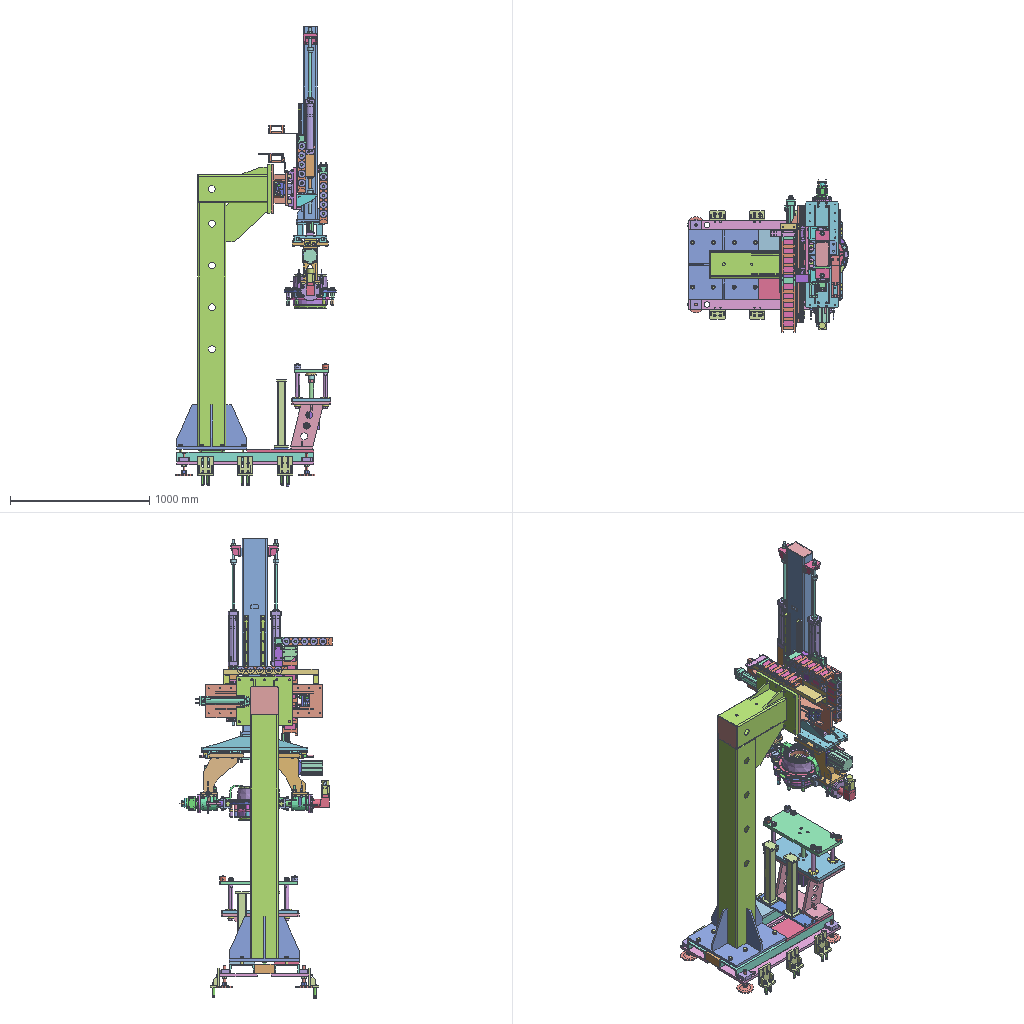Assembly | STEP file | 135 different items | 725 placed | box 1152 x 1093 x 3299 mm
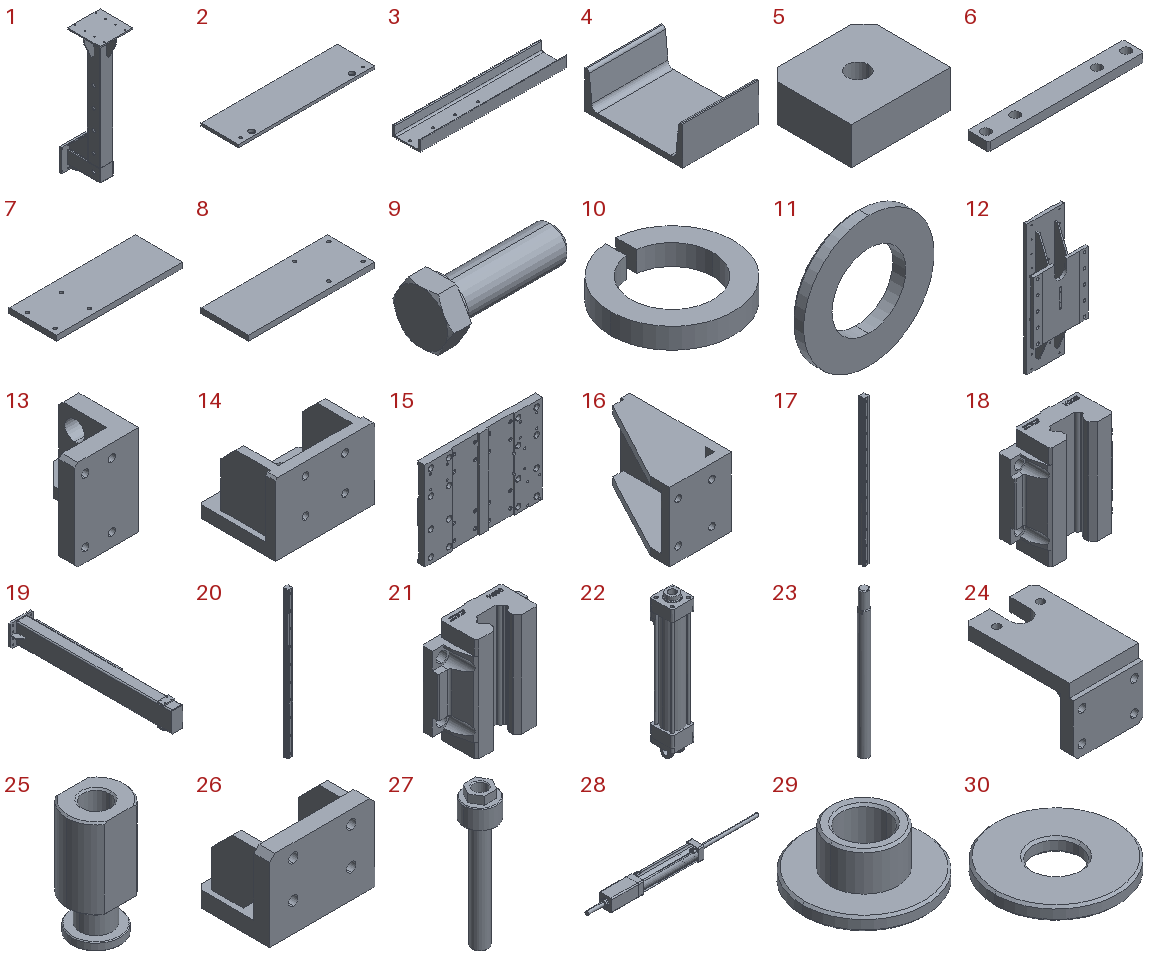Parts list (item | name | quantity | parent item | size | volume):
1 | YCD14007A-08.01.03 Column | x1 | in YCD14007A-08.01.00 Frame Component | 500 x 676 x 2044 mm | 25161780 mm3
2 | Base Plate | x2 | in YCD14007A-08.01.01 Base | 980 x 270 x 20 mm | 5232113 mm3
3 | 18# B Channel 980 (GB_INTERCHANGEABLE_PARTS_TM_SS 18X980)_GB_INTERCHANGEABLE_PARTS_TM_SS 18X980 | x2 | in YCD14007A-08.01.01 Base | 980 x 180 x 70 mm | 2864896 mm3
4 | 18# B Channel 140 (GB_INTERCHANGEABLE_PARTS_TM_SS 18X140)_GB_INTERCHANGEABLE_PARTS_TM_SS 18X140 | x2 | in YCD14007A-08.01.01 Base | 140 x 180 x 70 mm | 410063 mm3
5 | Thickening Block | x4 | in YCD14007A-08.01.01 Base | 80 x 70 x 30 mm | 157784 mm3
6 | Pad Plate | x1 | in YCD14007A-08.01.01 Base | 186 x 25 x 10 mm | 42619 mm3
7 | Small Pad Plate | x1 | in YCD14007A-08.01.01 Base | 480 x 180 x 20 mm | 1718952 mm3
8 | Small Pad Plate 1 | x1 | in YCD14007A-08.01.01 Base | 480 x 180 x 20 mm | 1718952 mm3
9 | Hex Head Bolt GB/T5783-2000 Fully Threaded M16x50 | x8 | in YCD14007A-08.01.00 Frame Component | 60 x 27.713 x 24 mm | 14933 mm3
10 | Spring Lock Washer GB/T93-1987 Standard Type (Assembly) 16x4.1 | x8 | in YCD14007A-08.01.00 Frame Component | 24.356 x 24.313 x 4.1 mm | 1031 mm3
11 | Flat Washer GB/T97.2-1985 Chamfered Type Grade A 16x3 | x8 | in YCD14007A-08.01.00 Frame Component | 30 x 3 x 30 mm | 1414 mm3
12 | YCD14007A-08.02.04-Lift Connecting Plate-A2 | x1 | in YCD14007A-08.02.00 Lifting Assembly | 350 x 120 x 840 mm | 6654945 mm3
13 | YCD14007A-08.02.07-Buffer Limit Seat-A3 | x1 | in YCD14007A-08.02.00 Lifting Assembly | 60 x 60 x 85 mm | 134562 mm3
14 | YCD14007A-08.02.08-Horizontal Cylinder Seat-A3 | x1 | in YCD14007A-08.02.00 Lifting Assembly | 100 x 77 x 72 mm | 177246 mm3
15 | YCD14007A-08.02.02-Adapter Plate-A3 | x1 | in YCD14007A-08.02.00 Lifting Assembly | 400 x 25 x 300 mm | 2208282 mm3
16 | YCD14007A-08.02.03-Lift Cylinder Seat-A3 | x2 | in YCD14007A-08.02.00 Lifting Assembly | 85 x 140.5 x 95 mm | 348010 mm3
17 | Slide Rail HGR35R840C | x2 | in Guide Rail Assembly | 34 x 29 x 840 mm | 682718 mm3
18 | HGW35CA20C+ZZ Slider | x4 | in Guide Rail Assembly | 100 x 40.5 x 112.7 mm | 283296 mm3
19 | YCD14007A-08.02.01 Slide | x1 | in YCD14007A-08.02.00 Lifting Assembly | 200 x 1406 x 200 mm | 5203563 mm3
20 | HGR30R-760 Slide Rail | x2 | in YCD14007A-08.02.00 Lifting Assembly | 28 x 26 x 760 mm | 438693 mm3
21 | HGW30 | x4 | in YCD14007A-08.02.00 Lifting Assembly | 90 x 36 x 97.7 mm | 189576 mm3
22 | MDBD50-250-A56 (Barrel) | x1 | in MBDB50-250-M9P | 65.01 x 74.997 x 403 mm | 1011039 mm3
23 | MDBD50-250-A56 (Rod) | x1 | in MBDB50-250-M9P | 20 x 20 x 309 mm | 94732 mm3
24 | YCD14007A-08.02.09-Horizontal Cylinder Connecting Plate-A3 | x1 | in YCD14007A-08.02.00 Lifting Assembly | 80 x 125 x 75 mm | 230135 mm3
25 | YCD14007A-08.02.11 Horizontal Cylinder Joint | x1 | in YCD14007A-08.02.00 Lifting Assembly | 36 x 30 x 71 mm | 47737 mm3
26 | YCD14007A-08.02.05-Lift Cylinder Connecting Plate-A3_Default<Machined> | x2 | in YCD14007A-08.02.00 Lifting Assembly | 100 x 70 x 75 mm | 222556 mm3
27 | YCD14007A-08.02.06-Extension Adjusting Rod-A4 | x4 | in YCD14007A-08.02.00 Lifting Assembly | 41 x 41 x 175 mm | 76364 mm3
28 | MDBB63-300-M9P_55_0_0 | x2 | in YCD14007A-08.02.00 Lifting Assembly | - | -
29 | YCD14007A-08.02.19 Lifting Cylinder Joint Modified | x3 | in YCD14007A-08.02.00 Lifting Assembly, Clamping Unit Assembly Left | 55 x 55 x 23 mm | 18397 mm3
30 | YCD14007A-08.02.19A Lifting Cylinder Joint Stop Plate Added | x3 | in YCD14007A-08.02.00 Lifting Assembly, Clamping Unit Assembly Left | 55 x 55 x 6 mm | 12037 mm3
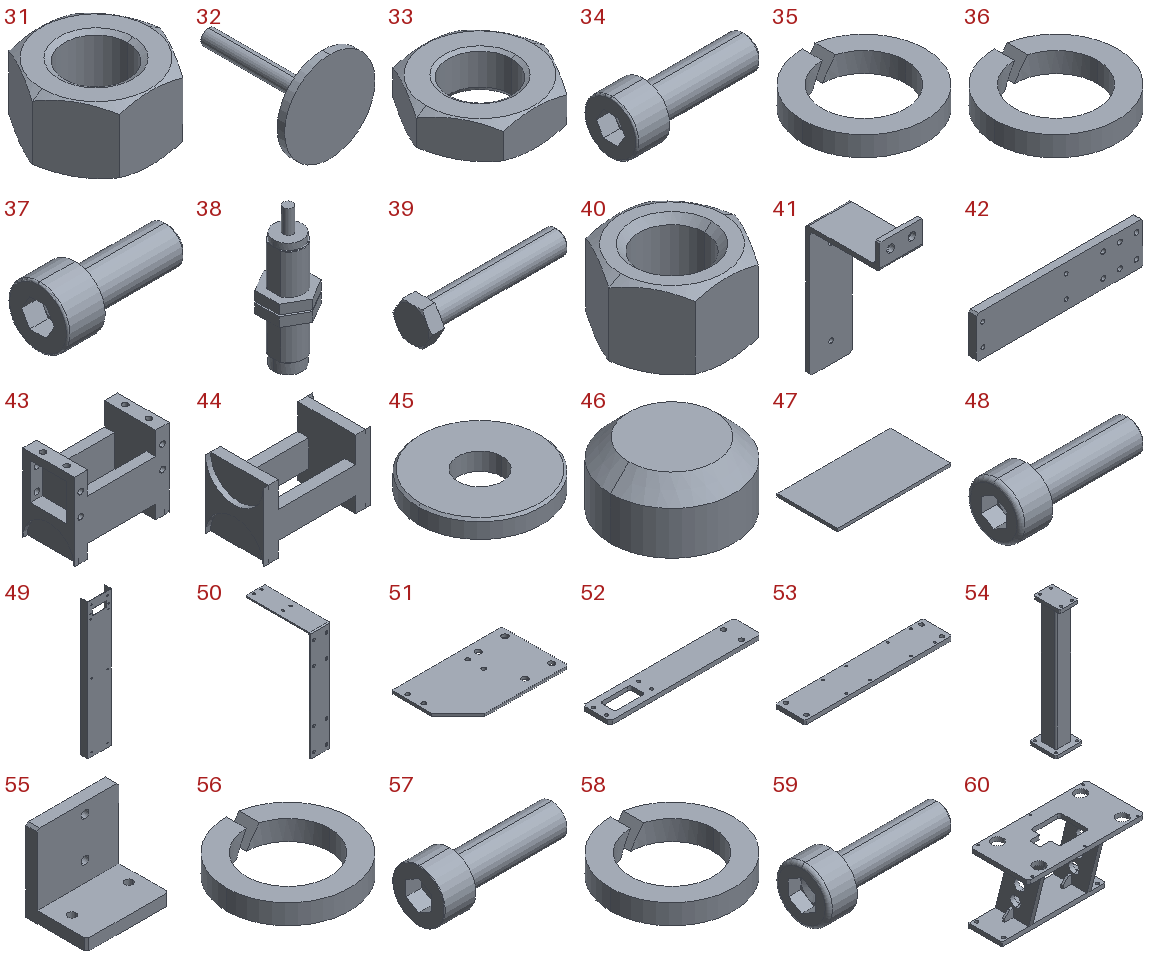31 | Hex Nut GB 6170-2000 M20 | x14 | in YCD14007A-08.02.00 Lifting Assembly, Clamping Unit Assembly Left | 34.641 x 30 x 18 mm | 9644 mm3
32 | Leveling Foot BF-20 | x4 | in Leveling Foot | 120 x 162 x 120 mm | 186987 mm3
33 | Hex Thin Nut M20_GB_FASTENER_NUT_STNAB B M20-N | x4 | in Leveling Foot | 34.641 x 30 x 10 mm | 5315 mm3
34 | Socket Head Cap Screw GB70.1-2000 M8X25 | x14 | in Turnover Unit Assembly, Clamping Unit Slide, Clamping Unit Assembly Left, Clamping Unit Assembly | 33 x 13 x 13 mm | 2167 mm3
35 | Spring Washer GB 93-87 10 | x32 | in Turnover Unit Assembly, Clamping Unit Assembly Left, Clamping Unit Assembly | 16.1 x 16.1 x 2.6 mm | 276.51 mm3
36 | Spring Washer GB 93-87 8 | x56 | in Turnover Unit Assembly, Clamping Unit Slide, Clamping Unit Assembly Left, Clamping Unit Assembly | 12.88 x 12.88 x 2.1 mm | 143.98 mm3
37 | Socket Head Cap Screw GB70.1-2000 M8X20 | x6 | in Turnover Unit Assembly | 28 x 13 x 13 mm | 1915 mm3
38 | Shock Absorber (SMC) RB2015 | x3 | in Turnover Unit Assembly, Clamping Unit Slide | 27 x 31.177 x 88.2 mm | 26039 mm3
39 | Hex Head Bolt GB5780-2000 M16(X1.5)X90_GB_FASTENER_BOLT_HHBFPT A M16X1.5X90-N | x3 | in Turnover Unit Assembly, Clamping Unit Slide | 99.82 x 27.332 x 23.67 mm | 22788 mm3
40 | Hex Nut GB 6170-2000 M16(X1.5)_GB_HEXAGON_TYPE10 M16X1.5-N | x6 | in Turnover Unit Assembly, Clamping Unit Slide | 27.713 x 24 x 16.4 mm | 5375 mm3
41 | Cable Carrier Channel Bracket | x3 | in Turnover Unit Assembly | 40 x 70 x 142 mm | 32841 mm3
42 | Cable Carrier Support Plate | x1 | in Cable Carrier Assembly | 180 x 8 x 45 mm | 63350 mm3
43 | Cable Carrier Part 1 | x4 | in Fully Enclosed Cable Carrier TLF-03 | 104 x 56 x 85 mm | 152286 mm3
44 | Cable Carrier Part 2 | x20 | in Fully Enclosed Cable Carrier TLF-03 | 104 x 56 x 66 mm | 123504 mm3
45 | Cable Carrier Part 3 | x40 | in Fully Enclosed Cable Carrier TLF-03 | 56 x 56 x 8 mm | 17104 mm3
46 | Cable Carrier Part 4 | x40 | in Fully Enclosed Cable Carrier TLF-03 | 20 x 20 x 10 mm | 2887 mm3
47 | Cable Carrier Seal Plate | x40 | in Fully Enclosed Cable Carrier TLF-03 | 75 x 40 x 2 mm | 6000 mm3
48 | Socket Head Cap Screw M5X16_GB_FASTENER_SCREWS_HSHCS M5X16-C | x8 | in Cable Carrier Assembly, Servo Motor SGMJV-04ADE6S and Reducer WPLE60-100 | 21 x 8.5 x 8.5 mm | 555.936 mm3
49 | Cable Carrier Channel | x1 | in Turnover Unit Assembly | 118 x 35 x 680 mm | 123926 mm3
50 | Cable Carrier Bracket | x1 | in Turnover Unit Assembly | 60 x 202 x 340 mm | 126408 mm3
51 | Cable Carrier Bracket 1 | x1 | in Turnover Unit Assembly | 165 x 100 x 4 mm | 61306 mm3
52 | Cable Carrier Bracket 2 | x1 | in Turnover Unit Assembly | 300 x 55 x 8 mm | 115449 mm3
53 | Fixed Base Plate | x1 | in Turnover Unit Assembly | 500 x 100 x 14 mm | 687217 mm3
54 | Cable Fixing Bracket | x2 | in Turnover Unit Assembly | 100 x 100 x 485 mm | 512449 mm3
55 | Cable Carrier Bracket 3 | x1 | in Turnover Unit Assembly | 72 x 53.558 x 72 mm | 81626 mm3
56 | Spring Washer GB 93-87 6 | x14 | in Turnover Unit Assembly, Clamping Unit Assembly Left, Clamping Unit Assembly | 9.88 x 9.88 x 1.6 mm | 64.217 mm3
57 | Socket Head Cap Screw GB/T70.1-2000 M6x20 | x14 | in Turnover Unit Assembly, YCD14007A-08.03.08 Left-Hand Mechanism.00, YCD14007A-08.03.07.00 Right-Hand Mechanism | 26 x 10 x 10 mm | 969.381 mm3
58 | Spring Washer 5_GB_FASTENER_WASHER_SW 5 | x8 | in Turnover Unit Assembly, Servo Motor SGMJV-04ADE6S and Reducer WPLE60-100 | 8 x 8 x 1.3 mm | 34.298 mm3
59 | _PreviewCfg | x2 | in Turnover Unit Assembly | 7.6 x 3 x 3 mm | 21.652 mm3
60 | Lifting Bracket | x1 | in Turnover Unit Assembly | 560 x 289.5 x 340 mm | 5840696 mm3
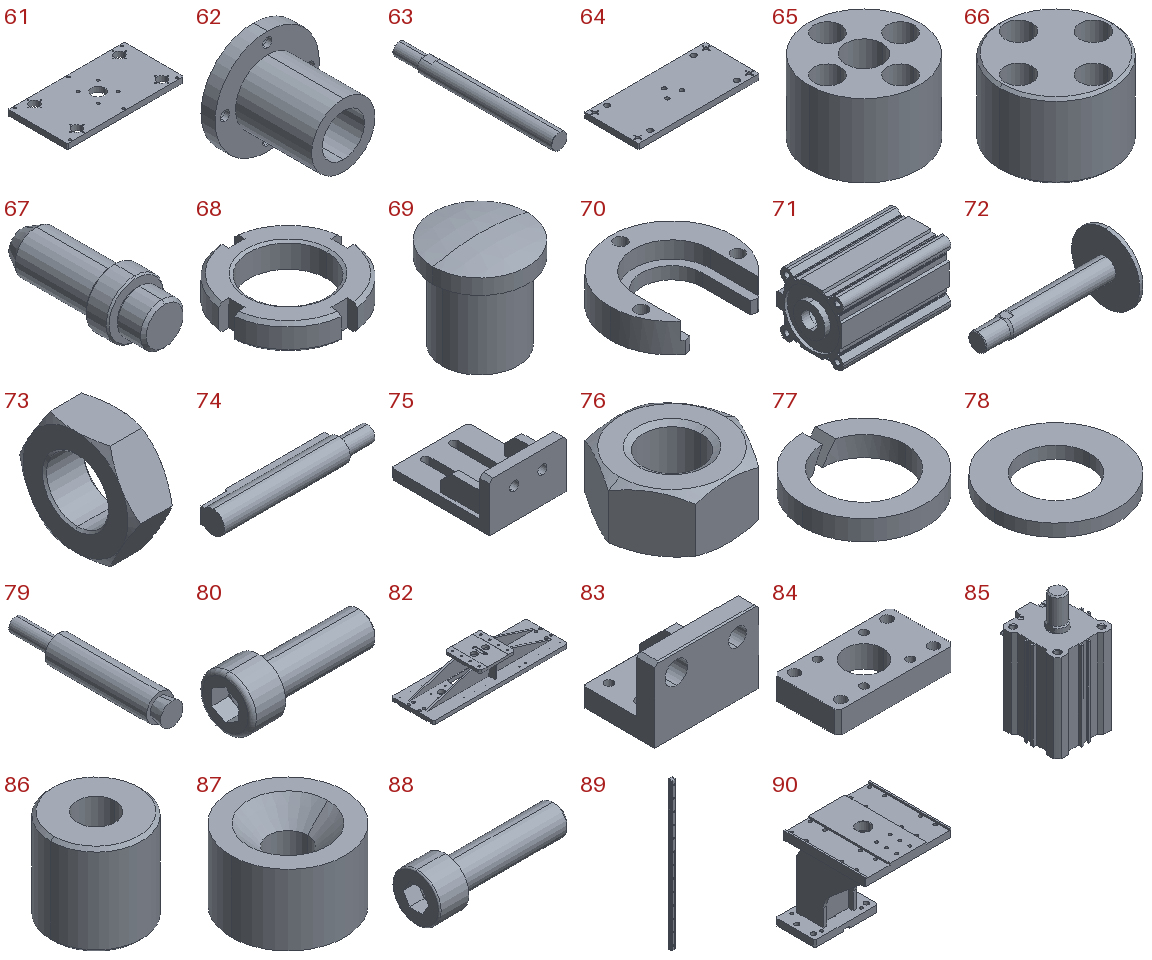61 | Lifting Base Plate | x1 | in Lift Positioning YCD14007A-17-0007-00 | 550 x 280 x 25 mm | 3578848 mm3
62 | LMF30UU | x4 | in Lift Positioning YCD14007A-17-0007-00 | 74 x 64 x 74 mm | 80630 mm3
63 | 30 Plain Shaft | x4 | in Lift Positioning YCD14007A-17-0007-00 | 30 x 305 x 30 mm | 202030 mm3
64 | Lifting Top Plate | x1 | in Lift Positioning YCD14007A-17-0007-00 | 560 x 250 x 25 mm | 3417013 mm3
65 | Locating Pin Seat | x2 | in Lift Positioning YCD14007A-17-0007-00 | 45 x 45 x 30 mm | 32214 mm3
66 | Locating Pin Seat | x2 | in Lift Positioning YCD14007A-17-0007-00 | 45 x 45 x 30 mm | 38603 mm3
67 | Locating Pin | x2 | in Lift Positioning YCD14007A-17-0007-00 | 20 x 50 x 20 mm | 9513 mm3
68 | Round Nut GB/T810-1988 M24x1.5 | x8 | in Lift Positioning YCD14007A-17-0007-00 | 37.67 x 37.67 x 8 mm | 4810 mm3
69 | Cylinder Joint | x1 | in Lift Positioning YCD14007A-17-0007-00 | 50 x 50 x 51 mm | 50075 mm3
70 | Cylinder Gland 2 | x1 | in Lift Positioning YCD14007A-17-0007-00 | 85 x 76.879 x 20 mm | 52737 mm3
71 | - | x1 | - | 205.5 x 123.5 x 117 mm | 1275384 mm3
72 | - | x1 | - | 193.5 x 100 x 100 mm | 165666 mm3
73 | NT-10(CQ2)_HI | x1 | - | 16 x 47.343 x 41 mm | 15625 mm3
74 | D_A96(CQ2L_100)_HI | x2 | - | 27 x 4.5 x 4 mm | 337.66 mm3
75 | Fixed Foot Plate | x6 | in Turnover Unit Assembly | 110 x 140 x 69 mm | 308717 mm3
76 | Nut M10-N_GB_FASTENER_NUT_SNAB1 M10-N | x12 | in Steel Expansion Bolt Assembly M10 | 18.475 x 16 x 8.4 mm | 1367 mm3
77 | Spring Washer SW 8_GB_FASTENER_WASHER_SW 8 | x12 | in Steel Expansion Bolt Assembly M10 | 12.88 x 12.88 x 2.1 mm | 143.98 mm3
78 | Flat Washer 10_GB_FASTENER_WASHER_SMWC 10 | x12 | in Steel Expansion Bolt Assembly M10 | 20 x 20 x 2 mm | 438.252 mm3
79 | Expansion Bolt M10X110 | x12 | in Steel Expansion Bolt Assembly M10 | 19.178 x 110 x 19.178 mm | 19450 mm3
80 | Socket Head Cap Screw M10X30-N_GB_FASTENER_SCREWS_HSHCS M10X30-N | x12 | in Turnover Unit Assembly | 40 x 16 x 16 mm | 4032 mm3
81 | Part 7 | x1 | in OP70 | - | -
82 | YCD14007A-08.03.02 Clamping Slide | x1 | in Clamping Unit Slide | 760 x 240 x 115 mm | 4249230 mm3
83 | YCD14007A-08.03.01 Buffer Limit Seat | x2 | in Clamping Unit Slide | 85 x 60 x 60 mm | 134508 mm3
84 | Locking Cylinder Mounting Plate | x1 | in Clamping Unit Slide | 100 x 56 x 19 mm | 79159 mm3
85 | A_CDQ2A40-40DM-A96V(0) | x2 | in Clamping Unit Slide, Latch Pin Assembly | 52 x 66.1 x 108 mm | 193246 mm3
86 | Locking Cylinder Joint | x1 | in Clamping Unit Slide | 30 x 30 x 30 mm | 16100 mm3
87 | Clamping Pad | x1 | in Clamping Unit Slide | 16 x 16 x 10 mm | 1679 mm3
88 | Socket Head Cap Screw GB70.1-2000 M8X30 | x38 | in Clamping Unit Slide, Clamping Unit Assembly Left, Clamping Unit Assembly | 38 x 13 x 13 mm | 2418 mm3
89 | HGR25R760C Guide Rail | x2 | in Clamping Unit Slide | 23 x 22 x 760 mm | 316727 mm3
90 | YCD14007A-08.03.06 Clamping Arm (Left) | x1 | in Clamping Unit Assembly Left | 260 x 306 x 295 mm | 2759054 mm3
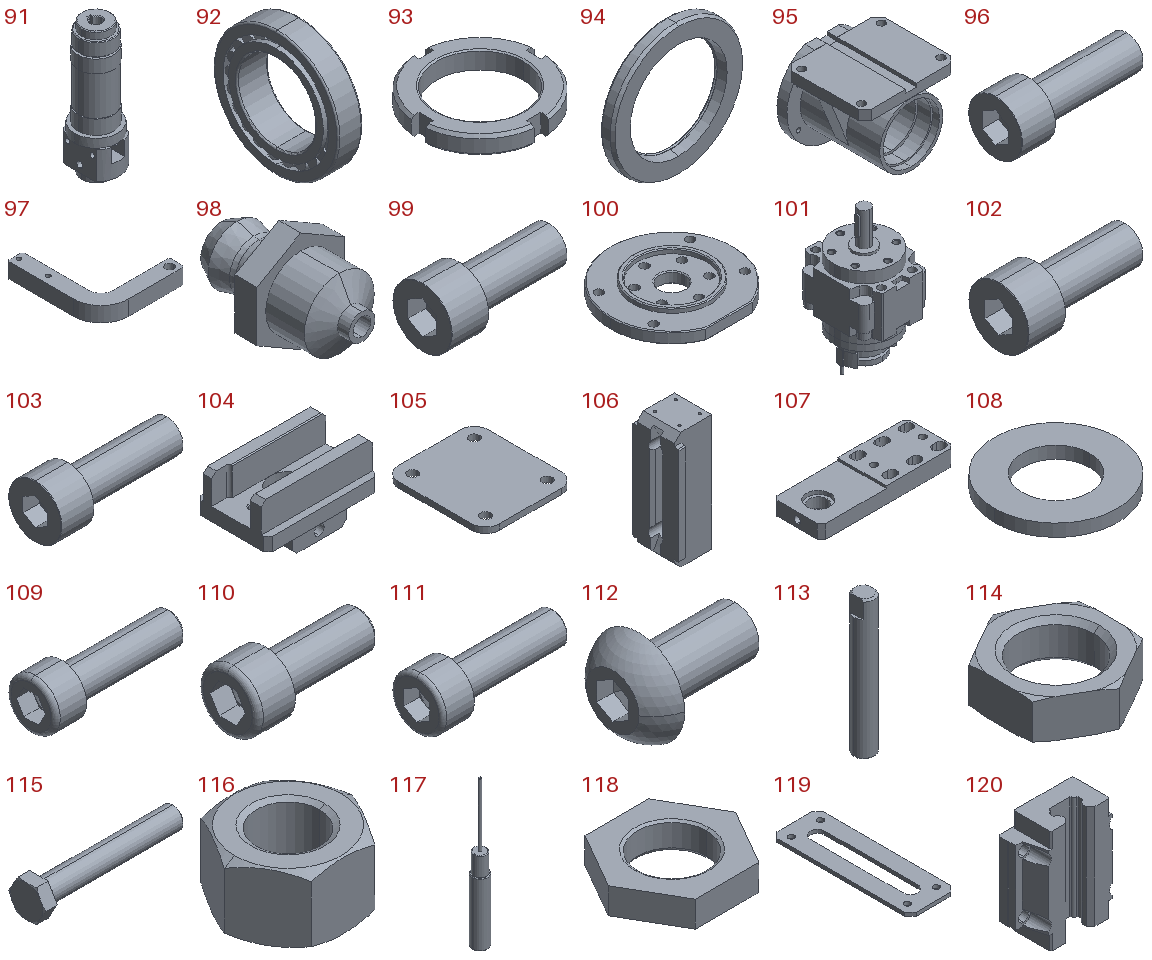91 | YCD14007A-08.03.08.01 Shaft (Cylinder) | x1 | in YCD14007A-08.03.08 Left-Hand Mechanism.00 | 60 x 65 x 185 mm | 338320 mm3
92 | Tapered Roller Bearing GB/T297-94 32010 | x4 | in YCD14007A-08.03.08 Left-Hand Mechanism.00, YCD14007A-08.03.07.00 Right-Hand Mechanism | 20 x 80 x 80 mm | 43880 mm3
93 | Round Nut GB/T810-1988 M48x1.5 | x2 | in YCD14007A-08.03.08 Left-Hand Mechanism.00 | 67.528 x 67.528 x 10 mm | 16343 mm3
94 | Lip Seal GB/T13871.1-2007 Type B B58_B1 | x3 | in YCD14007A-08.03.08 Left-Hand Mechanism.00, YCD14007A-08.03.07.00 Right-Hand Mechanism | 85 x 8 x 85 mm | 12919 mm3
95 | YCD14007A-08.03.07.04 Bearing Seat | x2 | in YCD14007A-08.03.08 Left-Hand Mechanism.00, YCD14007A-08.03.07.00 Right-Hand Mechanism | 140 x 135 x 130 mm | 675590 mm3
96 | Socket Head Cap Screw GB/T70.1-2000 M10x30 | x4 | in YCD14007A-08.03.08 Left-Hand Mechanism.00, YCD14007A-08.03.07.00 Right-Hand Mechanism | 40 x 16 x 16 mm | 4081 mm3
97 | YCD14007A-08.03.07.06 Limit Rod | x2 | in YCD14007A-08.03.08 Left-Hand Mechanism.00, YCD14007A-08.03.07.00 Right-Hand Mechanism | 100 x 112 x 18 mm | 57197 mm3
98 | Straight Grease Fitting JB/T7940.1-1995 8 | x2 | in YCD14007A-08.03.08 Left-Hand Mechanism.00, YCD14007A-08.03.07.00 Right-Hand Mechanism | 10 x 16 x 11.547 mm | 627.523 mm3
99 | Socket Head Cap Screw GB/T70.1-2000 M10x25 | x8 | in YCD14007A-08.03.08 Left-Hand Mechanism.00, YCD14007A-08.03.07.00 Right-Hand Mechanism | 35 x 16 x 16 mm | 3688 mm3
100 | YCD14007A-08.03.08.02 Adapter Flange (Cylinder) | x1 | in YCD14007A-08.03.08 Left-Hand Mechanism.00 | 135 x 130 x 17 mm | 160209 mm3
101 | CDRB1BW63-180S-S79_A_0 | x1 | in YCD14007A-08.03.08 Left-Hand Mechanism.00 | - | -
102 | Socket Head Cap Screw GB/T70.1-2000 M8x20 | x6 | in YCD14007A-08.03.08 Left-Hand Mechanism.00 | 28 x 13 x 13 mm | 1937 mm3
103 | Socket Head Cap Screw GB/T70.1-2000 M8x25 | x8 | in YCD14007A-08.03.08 Left-Hand Mechanism.00, YCD14007A-08.03.07.00 Right-Hand Mechanism | 33 x 13 x 13 mm | 2189 mm3
104 | YCD14007A-08.03.07.08 Gripper Seat | x2 | in YCD14007A-08.03.08 Left-Hand Mechanism.00, YCD14007A-08.03.07.00 Right-Hand Mechanism | 125 x 80 x 67 mm | 253618 mm3
105 | YCD14007A-08.03.08.05 Engraving Plate | x2 | in Clamping Unit Assembly Left, Clamping Unit Assembly | 32 x 36 x 2 mm | 2184 mm3
106 | Nylon Claw M20 | x2 | in Clamping Unit Assembly Left, Clamping Unit Assembly | 40 x 50 x 125 mm | 179842 mm3
107 | YCD14007A-08.02.17 Lock Plate | x1 | in Clamping Unit Assembly Left | 165 x 60 x 20 mm | 154509 mm3
108 | Flat Washer GB 95-85 10_GB_FASTENER_WASHER_SMWC 10 | x4 | in Clamping Unit Assembly Left | 20 x 20 x 2 mm | 438.252 mm3
109 | Socket Head Cap Screw GB70.1-2000 M10X35 | x12 | in Clamping Unit Assembly Left, Clamping Unit Assembly | 45 x 16 x 16 mm | 4402 mm3
110 | Socket Head Cap Screw GB70.1-2000 M10X25 | x4 | in Clamping Unit Assembly Left, Clamping Unit Assembly | 35 x 16 x 16 mm | 3616 mm3
111 | Socket Set Screw GB79-2000 M6X20_GB_FASTENER_SCREWS_HSHCS M6X20-N | x8 | in Clamping Unit Assembly Left, Clamping Unit Assembly | 26 x 10 x 10 mm | 958.089 mm3
112 | Socket Button Head Screw M3X6-N_GB_SOCKET_TYPE7 M3X6-N | x8 | in Clamping Unit Assembly Left, Clamping Unit Assembly | 7.65 x 5.7 x 5.7 mm | 68.602 mm3
113 | YCD14007A-08-03.07.07 Sensing Rod | x2 | in Clamping Unit Assembly Left, YCD14007A-08.03.07.00 Right-Hand Mechanism | 12 x 12 x 82 mm | 9083 mm3
114 | Hex Nut GB/T6172.1-2000 Grade A and B M12 | x4 | in Clamping Unit Assembly Left, YCD14007A-08.03.07.00 Right-Hand Mechanism, Clamping Unit Assembly | 17.386 x 20.03 x 6 mm | 858.5 mm3
115 | Hex Head Bolt GB5780-2000 M16X100 | x4 | in Clamping Unit Assembly Left, Clamping Unit Assembly | 110 x 27.713 x 24 mm | 24997 mm3
116 | Hex Nut GB 6170-2000 M16 | x8 | in Clamping Unit Assembly Left, Clamping Unit Assembly | 27.713 x 24 x 14.8 mm | 5071 mm3
117 | YB Inductive Proximity Switch | x6 | in Proximity Switch Assembly, Clamping Unit Assembly Left, Clamping Unit Assembly | 12 x 12 x 115 mm | 6984 mm3
118 | Fine-Thread Nut M12X1_GB_FASTENER_NUT_STNABTT M12X1.25-N | x14 | in Proximity Switch Assembly, Clamping Unit Assembly Left, Clamping Unit Assembly | 19.63 x 17 x 4 mm | 641.848 mm3
119 | Mounting Plate | x1 | in Proximity Switch Assembly | 40 x 120 x 3 mm | 10646 mm3
120 | HGW25CA0C+ZZ | x8 | in Clamping Unit Assembly Left, Clamping Unit Assembly | 70 x 30.5 x 82 mm | 109676 mm3
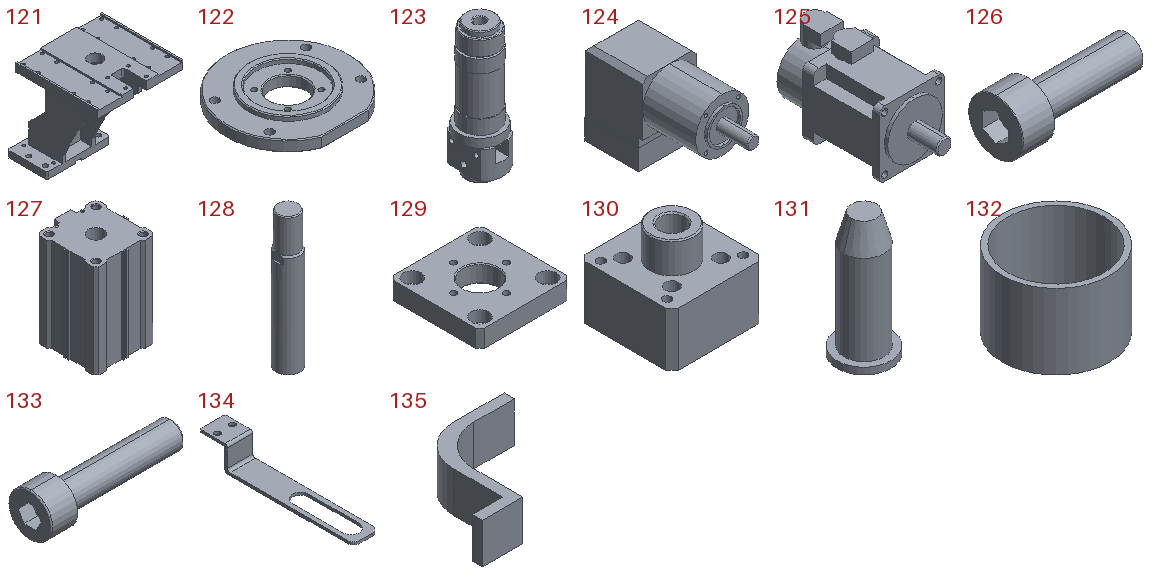121 | YCD14007A-08.03.03 Clamping Arm (Right) | x1 | in Clamping Unit Assembly | 260 x 306 x 295 mm | 2644303 mm3
122 | YCD14007A-08.03.07.05 Adapter Flange (Motor) | x1 | in YCD14007A-08.03.07.00 Right-Hand Mechanism | 135 x 130 x 17 mm | 158776 mm3
123 | YCD14007A-08.03.07.03 Shaft (Motor) | x1 | in YCD14007A-08.03.07.00 Right-Hand Mechanism | 60 x 65 x 185 mm | 341019 mm3
124 | Right-Angle Reducer WPLE60-100 | x1 | in Servo Motor SGMJV-04ADE6S and Reducer WPLE60-100 | 60.05 x 160.025 x 93 mm | 504170 mm3
125 | SGMJV-04ADE6S (Yaskawa Servo 0.4KW) | x1 | in Servo Motor SGMJV-04ADE6S and Reducer WPLE60-100 | 60 x 129 x 73 mm | 298777 mm3
126 | Socket Head Cap Screw GB/T70.1-2000 M5x16 | x4 | in YCD14007A-08.03.07.00 Right-Hand Mechanism | 21 x 8.5 x 8.5 mm | 561.928 mm3
127 | A_CDQ2A80-100DM-F9NV (Barrel) | x1 | in CDQ2A80-100DMZ | 98 x 108.4 x 153.5 mm | 1262277 mm3
128 | A_CDQ2A80-100DM-F9NV (Rod) | x1 | in CDQ2A80-100DMZ | 25 x 25 x 144.5 mm | 66720 mm3
129 | Clamping Cylinder Mounting Plate | x1 | in Clamping Unit Assembly | 104 x 104 x 20 mm | 167084 mm3
130 | YCD14007A-08.02.14 Latch Cylinder Seat | x1 | in Latch Pin Assembly | 76 x 76 x 69 mm | 233677 mm3
131 | YCD14007A-08.02.15 Latch Cylinder Joint | x1 | in Latch Pin Assembly | 24 x 24 x 55 mm | 9061 mm3
132 | Oil-Free Bushing JH-B-18-14 | x2 | in Latch Pin Assembly | 20 x 20 x 14 mm | 835.664 mm3
133 | Socket Head Cap Screw GB70.1-2000 M8X35 | x4 | in Clamping Unit Assembly | 43 x 13 x 13 mm | 2669 mm3
134 | Proximity Switch Bracket | x2 | in Clamping Unit Assembly | 20 x 122 x 20 mm | 4207 mm3
135 | Pressure Rod | x2 | in Turnover Unit Assembly | 120 x 98.5 x 40 mm | 83400 mm3
Placements (level | parent | child | x y z in mm | rotation matrix by rows), first 157 of 765 lines:
1 | Turnover Unit Assembly | YCD14007A-08.01.00 Frame Component | -651.902 -316.685 -698.035 | 0 1 0 1 0 0 0 0 -1
2 | YCD14007A-08.01.00 Frame Component | YCD14007A-08.01.03 Column | -109.585 -100.226 1002.0 | 1 0 0 0 1 0 0 0 1
2 | YCD14007A-08.01.00 Frame Component | YCD14007A-08.01.01 Base | -386.402 100.206 1132.0 | 0 1 0 1 0 0 0 0 -1
3 | YCD14007A-08.01.01 Base | Base Plate | 39.567 91.817 -0.0 | 1 0 0 0 1 0 0 0 1
3 | YCD14007A-08.01.01 Base | 18# B Channel 980 (GB_INTERCHANGEABLE_PARTS_TM_SS 18X980)_GB_INTERCHANGEABLE_PARTS_TM_SS 18X980 | -450.433 116.817 90.0 | 1 0 0 0 -1 0 0 0 -1
3 | YCD14007A-08.01.01 Base | 18# B Channel 980 (GB_INTERCHANGEABLE_PARTS_TM_SS 18X980)_GB_INTERCHANGEABLE_PARTS_TM_SS 18X980 | -450.433 436.817 90.0 | 1 0 0 0 -1 0 0 0 -1
3 | YCD14007A-08.01.01 Base | Base Plate | 39.567 461.817 20.0 | 1 0 0 0 -1 0 0 0 -1
3 | YCD14007A-08.01.01 Base | 18# B Channel 140 (GB_INTERCHANGEABLE_PARTS_TM_SS 18X140)_GB_INTERCHANGEABLE_PARTS_TM_SS 18X140 | -360.433 206.816 90.0 | 0 1 0 1 0 0 0 0 -1
3 | YCD14007A-08.01.01 Base | 18# B Channel 140 (GB_INTERCHANGEABLE_PARTS_TM_SS 18X140)_GB_INTERCHANGEABLE_PARTS_TM_SS 18X140 | 439.567 206.816 90.0 | 0 1 0 1 0 0 0 0 -1
3 | YCD14007A-08.01.01 Base | Thickening Block | -400.433 561.817 20.0 | 0.9999 0.01671 0 -0.01671 0.9999 0 0 0 1
3 | YCD14007A-08.01.01 Base | Thickening Block | 479.567 561.817 50.0 | -1 0 0 0 1 0 0 0 -1
3 | YCD14007A-08.01.01 Base | Thickening Block | -400.433 -8.184 50.0 | 1 0 0 0 -1 0 0 0 -1
3 | YCD14007A-08.01.01 Base | Thickening Block | 479.567 -8.184 50.0 | 1 0 0 0 -1 0 0 0 -1
3 | YCD14007A-08.01.01 Base | Pad Plate | -200.433 276.817 90.0 | 1 0 0 0 1 0 0 0 1
3 | YCD14007A-08.01.01 Base | Small Pad Plate | 289.567 116.817 90.0 | -1 0 0 0 -1 0 0 0 1
3 | YCD14007A-08.01.01 Base | Small Pad Plate 1 | 289.567 436.817 90.0 | 1 0 0 0 1 0 0 0 1
2 | YCD14007A-08.01.00 Frame Component | Hex Head Bolt GB/T5783-2000 Fully Threaded M16x50 | 50.415 -325.226 984.9 | 0 0 -1 0 1 0 1 0 0
2 | YCD14007A-08.01.00 Frame Component | Spring Lock Washer GB/T93-1987 Standard Type (Assembly) 16x4.1 | 50.415 -325.226 994.9 | 1 0 0 0 1 0 0 0 1
2 | YCD14007A-08.01.00 Frame Component | Flat Washer GB/T97.2-1985 Chamfered Type Grade A 16x3 | 50.415 -325.226 1010.644 | 1 0 0 0 0 1 0 -1 -0
2 | YCD14007A-08.01.00 Frame Component | Spring Lock Washer GB/T93-1987 Standard Type (Assembly) 16x4.1 | -269.585 -325.226 994.9 | 1 0 0 0 1 0 0 0 1
2 | YCD14007A-08.01.00 Frame Component | Spring Lock Washer GB/T93-1987 Standard Type (Assembly) 16x4.1 | 50.415 -175.226 994.9 | 1 0 0 0 1 0 0 0 1
2 | YCD14007A-08.01.00 Frame Component | Spring Lock Washer GB/T93-1987 Standard Type (Assembly) 16x4.1 | -269.585 -175.226 994.9 | 1 0 0 0 1 0 0 0 1
2 | YCD14007A-08.01.00 Frame Component | Spring Lock Washer GB/T93-1987 Standard Type (Assembly) 16x4.1 | 50.415 -25.226 994.9 | 1 0 0 0 1 0 0 0 1
2 | YCD14007A-08.01.00 Frame Component | Spring Lock Washer GB/T93-1987 Standard Type (Assembly) 16x4.1 | -269.585 -25.226 994.9 | 1 0 0 0 1 0 0 0 1
2 | YCD14007A-08.01.00 Frame Component | Spring Lock Washer GB/T93-1987 Standard Type (Assembly) 16x4.1 | 50.415 124.774 994.9 | 1 0 0 0 1 0 0 0 1
2 | YCD14007A-08.01.00 Frame Component | Spring Lock Washer GB/T93-1987 Standard Type (Assembly) 16x4.1 | -269.585 124.774 994.9 | 1 0 0 0 1 0 0 0 1
2 | YCD14007A-08.01.00 Frame Component | Flat Washer GB/T97.2-1985 Chamfered Type Grade A 16x3 | -269.585 -325.226 1010.644 | 1 0 0 0 0 1 0 -1 -0
2 | YCD14007A-08.01.00 Frame Component | Flat Washer GB/T97.2-1985 Chamfered Type Grade A 16x3 | 50.415 -175.226 1010.644 | 1 0 0 0 0 1 0 -1 -0
2 | YCD14007A-08.01.00 Frame Component | Flat Washer GB/T97.2-1985 Chamfered Type Grade A 16x3 | -269.585 -175.226 1010.644 | 1 0 0 0 0 1 0 -1 -0
2 | YCD14007A-08.01.00 Frame Component | Flat Washer GB/T97.2-1985 Chamfered Type Grade A 16x3 | 50.415 -25.226 1010.644 | 1 0 0 0 0 1 0 -1 -0
2 | YCD14007A-08.01.00 Frame Component | Flat Washer GB/T97.2-1985 Chamfered Type Grade A 16x3 | -269.585 -25.226 1010.644 | 1 0 0 0 0 1 0 -1 -0
2 | YCD14007A-08.01.00 Frame Component | Flat Washer GB/T97.2-1985 Chamfered Type Grade A 16x3 | 50.415 124.774 1010.644 | 1 0 0 0 0 1 0 -1 -0
2 | YCD14007A-08.01.00 Frame Component | Flat Washer GB/T97.2-1985 Chamfered Type Grade A 16x3 | -269.585 124.774 1010.644 | 1 0 0 0 0 1 0 -1 -0
2 | YCD14007A-08.01.00 Frame Component | Hex Head Bolt GB/T5783-2000 Fully Threaded M16x50 | -269.585 -325.226 984.9 | 0 0 -1 0 1 0 1 0 0
2 | YCD14007A-08.01.00 Frame Component | Hex Head Bolt GB/T5783-2000 Fully Threaded M16x50 | 50.415 -175.226 984.9 | 0 0 -1 0 1 0 1 0 0
2 | YCD14007A-08.01.00 Frame Component | Hex Head Bolt GB/T5783-2000 Fully Threaded M16x50 | -269.585 -175.226 984.9 | 0 0 -1 0 1 0 1 0 0
2 | YCD14007A-08.01.00 Frame Component | Hex Head Bolt GB/T5783-2000 Fully Threaded M16x50 | 50.415 -25.226 984.9 | 0 0 -1 0 1 0 1 0 0
2 | YCD14007A-08.01.00 Frame Component | Hex Head Bolt GB/T5783-2000 Fully Threaded M16x50 | -269.585 -25.226 984.9 | 0 0 -1 0 1 0 1 0 0
2 | YCD14007A-08.01.00 Frame Component | Hex Head Bolt GB/T5783-2000 Fully Threaded M16x50 | 50.415 124.774 984.9 | 0 0 -1 0 1 0 1 0 0
2 | YCD14007A-08.01.00 Frame Component | Hex Head Bolt GB/T5783-2000 Fully Threaded M16x50 | -269.585 124.774 984.9 | 0 0 -1 0 1 0 1 0 0
1 | Turnover Unit Assembly | YCD14007A-08.02.00 Lifting Assembly | -1012.217 -846.27 -316.467 | -0.8169 0.5767 0 0 0 -1 -0.5767 -0.8169 -0
2 | YCD14007A-08.02.00 Lifting Assembly | YCD14007A-08.02.04-Lift Connecting Plate-A2 | -918.783 78.885 0.0 | -0.5767 -0.8169 0 -0.8169 0.5767 0 0 0 -1
2 | YCD14007A-08.02.00 Lifting Assembly | YCD14007A-08.02.07-Buffer Limit Seat-A3 | -890.221 110.745 -132.161 | 0 0.8169 -0.5767 0 -0.5767 -0.8169 -1 0 -0
2 | YCD14007A-08.02.00 Lifting Assembly | YCD14007A-08.02.08-Horizontal Cylinder Seat-A3 | -879.161 50.914 -515.5 | 0.5767 0.8169 0 0.8169 -0.5767 0 0 0 -1
2 | YCD14007A-08.02.00 Lifting Assembly | YCD14007A-08.02.02-Adapter Plate-A3 | -881.701 236.317 -489.348 | 0 0.8169 0.5767 0 -0.5767 0.8169 1 0 0
2 | YCD14007A-08.02.00 Lifting Assembly | YCD14007A-08.02.03-Lift Cylinder Seat-A3 | -915.269 231.249 -594.348 | -0.5767 -0.8169 0 -0.8169 0.5767 0 0 0 -1
2 | YCD14007A-08.02.00 Lifting Assembly | YCD14007A-08.02.03-Lift Cylinder Seat-A3 | -915.269 231.249 -289.348 | -0.5767 -0.8169 0 -0.8169 0.5767 0 0 0 -1
2 | YCD14007A-08.02.00 Lifting Assembly | Guide Rail Assembly | -1028.88 -38.564 -420.0 | -0.5767 -0.8169 0 -0.8169 0.5767 0 0 0 -1
3 | Guide Rail Assembly | Slide Rail HGR35R840C | -69.443 -2.709 420.0 | 1 0 0 0 1 0 0 0 1
3 | Guide Rail Assembly | HGW35CA20C+ZZ Slider | -69.443 11.791 218.148 | 1 0 0 0 1 0 0 0 1
3 | Guide Rail Assembly | HGW35CA20C+ZZ Slider | -69.443 11.791 -79.452 | 1 0 0 0 1 0 0 0 1
2 | YCD14007A-08.02.00 Lifting Assembly | Guide Rail Assembly | -925.071 108.487 -420.0 | -0.5767 -0.8169 0 -0.8169 0.5767 0 0 0 -1
3 | Guide Rail Assembly | Slide Rail HGR35R840C | -69.443 -2.709 420.0 | 1 0 0 0 1 0 0 0 1
3 | Guide Rail Assembly | HGW35CA20C+ZZ Slider | -69.443 11.791 218.148 | 1 0 0 0 1 0 0 0 1
3 | Guide Rail Assembly | HGW35CA20C+ZZ Slider | -69.443 11.791 -79.452 | 1 0 0 0 1 0 0 0 1
2 | YCD14007A-08.02.00 Lifting Assembly | YCD14007A-08.02.01 Slide | -925.596 364.007 -589.348 | 0.8169 0.5767 0 -0.5767 0.8169 0 0 0 1
2 | YCD14007A-08.02.00 Lifting Assembly | HGR30R-760 Slide Rail | -910.626 258.633 -549.348 | 0 0.8169 -0.5767 0 -0.5767 -0.8169 -1 0 -0
2 | YCD14007A-08.02.00 Lifting Assembly | HGW30 | -1045.828 44.572 -549.348 | 0 0.8169 -0.5767 0 -0.5767 -0.8169 -1 0 -0
2 | YCD14007A-08.02.00 Lifting Assembly | HGW30 | -928.985 210.085 -549.348 | 0 0.8169 -0.5767 0 -0.5767 -0.8169 -1 0 -0
2 | YCD14007A-08.02.00 Lifting Assembly | HGR30R-760 Slide Rail | -910.626 258.633 -429.348 | 0 0.8169 -0.5767 0 -0.5767 -0.8169 -1 0 -0
2 | YCD14007A-08.02.00 Lifting Assembly | HGW30 | -1045.828 44.572 -429.348 | 0 0.8169 -0.5767 0 -0.5767 -0.8169 -1 0 -0
2 | YCD14007A-08.02.00 Lifting Assembly | HGW30 | -928.985 210.085 -429.348 | 0 0.8169 -0.5767 0 -0.5767 -0.8169 -1 0 -0
2 | YCD14007A-08.02.00 Lifting Assembly | MBDB50-250-M9P | -914.55 -16.727 -715.001 | -0.5767 0.8169 0 -0.8169 -0.5767 0 0 0 1
3 | MBDB50-250-M9P | MDBD50-250-A56 (Barrel) | -75.668 -3.348 187.501 | 1 0 0 0 1 0 0 0 1
3 | MBDB50-250-M9P | MDBD50-250-A56 (Rod) | -75.668 -3.348 219.653 | -0.6044 0.7967 0 -0.7967 -0.6044 0 0 0 1
2 | YCD14007A-08.02.00 Lifting Assembly | YCD14007A-08.02.09-Horizontal Cylinder Connecting Plate-A3 | -904.895 69.08 -396.848 | 0.5767 0.8169 0 0.8169 -0.5767 0 0 0 -1
2 | YCD14007A-08.02.00 Lifting Assembly | YCD14007A-08.02.11 Horizontal Cylinder Joint | -873.647 47.021 -391.348 | -0.6292 0.7773 0 0.7773 0.6292 0 0 0 -1
2 | YCD14007A-08.02.00 Lifting Assembly | YCD14007A-08.02.05-Lift Cylinder Connecting Plate-A3_Default<Machined> | -1689.456 -718.037 -351.848 | -0.8169 0 0.5767 0.5767 0 0.8169 0 1 -0
2 | YCD14007A-08.02.00 Lifting Assembly | YCD14007A-08.02.05-Lift Cylinder Connecting Plate-A3_Default<Machined> | -1689.456 -718.037 -626.848 | 0.8169 0 0.5767 -0.5767 0 0.8169 0 -1 0
2 | YCD14007A-08.02.00 Lifting Assembly | YCD14007A-08.02.06-Extension Adjusting Rod-A4 | -1642.333 -652.153 -336.848 | 0.8166 -0.0243 0.5767 -0.5765 0.01716 0.8169 -0.02975 -0.9996 -0
2 | YCD14007A-08.02.00 Lifting Assembly | YCD14007A-08.02.06-Extension Adjusting Rod-A4 | -1642.333 -652.153 -641.848 | 0.1425 0.8044 0.5767 -0.1006 -0.5679 0.8169 0.9847 -0.1744 -0
2 | YCD14007A-08.02.00 Lifting Assembly | MDBB63-300-M9P_55_0_0 | -1201.146 -27.19 -336.848 | -0.5767 0 -0.8169 -0.8169 0 0.5767 0 1 -0
2 | YCD14007A-08.02.00 Lifting Assembly | MDBB63-300-M9P_55_0_0 | -1201.146 -27.19 -641.848 | -0.5767 0 0.8169 -0.8169 0 -0.5767 0 -1 0
2 | YCD14007A-08.02.00 Lifting Assembly | YCD14007A-08.02.06-Extension Adjusting Rod-A4 | -1036.782 205.639 -641.848 | 0.1342 -0.8059 -0.5767 -0.09471 0.5689 -0.8169 0.9864 0.1642 0
2 | YCD14007A-08.02.00 Lifting Assembly | YCD14007A-08.02.06-Extension Adjusting Rod-A4 | -1036.782 205.639 -336.848 | -0.7262 -0.3742 -0.5767 0.5127 0.2642 -0.8169 0.458 -0.8889 0
2 | YCD14007A-08.02.00 Lifting Assembly | YCD14007A-08.02.19 Lifting Cylinder Joint Modified | -1030.15 215.034 -641.848 | -0.1862 0.7955 0.5767 0.1314 -0.5615 0.8169 0.9737 0.2279 -0
2 | YCD14007A-08.02.00 Lifting Assembly | YCD14007A-08.02.19A Lifting Cylinder Joint Stop Plate Added | -1021.787 226.88 -641.848 | 0.6674 -0.4711 -0.5767 -0.4711 0.3326 -0.8169 0.5767 0.8169 -0
2 | YCD14007A-08.02.00 Lifting Assembly | Hex Nut GB 6170-2000 M20 | -1697.698 -730.58 -336.848 | 0.8162 0.03372 0.5767 -0.5762 -0.0238 0.8169 0.04127 -0.9991 -0
2 | YCD14007A-08.02.00 Lifting Assembly | Hex Nut GB 6170-2000 M20 | -1678.666 -703.621 -336.848 | 0.8162 0.03372 0.5767 -0.5762 -0.0238 0.8169 0.04127 -0.9991 -0
2 | YCD14007A-08.02.00 Lifting Assembly | Hex Nut GB 6170-2000 M20 | -1014.867 236.683 -641.848 | 0.8162 0.03372 0.5767 -0.5762 -0.0238 0.8169 0.04127 -0.9991 -0
2 | YCD14007A-08.02.00 Lifting Assembly | Hex Nut GB 6170-2000 M20 | -1004.486 251.388 -641.848 | 0.8162 0.03372 0.5767 -0.5762 -0.0238 0.8169 0.04127 -0.9991 -0
2 | YCD14007A-08.02.00 Lifting Assembly | Hex Nut GB 6170-2000 M20 | -1014.867 236.683 -336.848 | 0.8162 0.03372 0.5767 -0.5762 -0.0238 0.8169 0.04127 -0.9991 -0
2 | YCD14007A-08.02.00 Lifting Assembly | Hex Nut GB 6170-2000 M20 | -1004.486 251.388 -336.848 | 0.8162 0.03372 0.5767 -0.5762 -0.0238 0.8169 0.04127 -0.9991 -0
2 | YCD14007A-08.02.00 Lifting Assembly | Hex Nut GB 6170-2000 M20 | -1697.698 -730.58 -641.848 | 0.8136 0.07426 0.5767 -0.5743 -0.05242 0.8169 0.0909 -0.9959 -0
2 | YCD14007A-08.02.00 Lifting Assembly | Hex Nut GB 6170-2000 M20 | -1678.666 -703.621 -641.848 | 0.8162 0.03372 0.5767 -0.5762 -0.0238 0.8169 0.04127 -0.9991 -0
2 | YCD14007A-08.02.00 Lifting Assembly | YCD14007A-08.02.19 Lifting Cylinder Joint Modified | -1030.15 215.034 -336.848 | 0.1862 0.7955 0.5767 -0.1314 -0.5615 0.8169 0.9737 -0.2279 0
2 | YCD14007A-08.02.00 Lifting Assembly | YCD14007A-08.02.19A Lifting Cylinder Joint Stop Plate Added | -1021.787 226.88 -336.848 | 0.6674 -0.4711 0.5767 -0.4711 0.3326 0.8169 -0.5767 -0.8169 -0
2 | YCD14007A-08.02.00 Lifting Assembly | Hex Nut GB 6170-2000 M20 | -1025.249 221.976 -336.848 | 0.8162 0.03372 -0.5767 -0.5762 -0.0238 -0.8169 -0.04127 0.9991 -0
2 | YCD14007A-08.02.00 Lifting Assembly | Hex Nut GB 6170-2000 M20 | -1014.868 236.681 -336.848 | 0.8162 0.03372 -0.5767 -0.5762 -0.0238 -0.8169 -0.04127 0.9991 -0
1 | Turnover Unit Assembly | Leveling Foot | -72.128 -711.27 -1910.035 | 1 0 0 0 0 -1 0 1 0
2 | Leveling Foot | Leveling Foot BF-20 | -0.0 -0.0 -0.0 | -1 0 0 0 1 0 0 0 -1
2 | Leveling Foot | Hex Thin Nut M20_GB_FASTENER_NUT_STNAB B M20-N | -0.0 80.0 -0.0 | 1 0 0 0 0 1 0 -1 0
1 | Turnover Unit Assembly | Leveling Foot | -952.128 -711.27 -1910.035 | 1 0 0 0 0 -1 0 1 0
2 | Leveling Foot | Leveling Foot BF-20 | -0.0 -0.0 -0.0 | -1 0 0 0 1 0 0 0 -1
2 | Leveling Foot | Hex Thin Nut M20_GB_FASTENER_NUT_STNAB B M20-N | -0.0 80.0 -0.0 | 1 0 0 0 0 1 0 -1 0
1 | Turnover Unit Assembly | Leveling Foot | -72.128 -141.27 -1910.035 | 1 0 0 0 0 -1 0 1 0
2 | Leveling Foot | Leveling Foot BF-20 | -0.0 -0.0 -0.0 | -1 0 0 0 1 0 0 0 -1
2 | Leveling Foot | Hex Thin Nut M20_GB_FASTENER_NUT_STNAB B M20-N | -0.0 80.0 -0.0 | 1 0 0 0 0 1 0 -1 0
1 | Turnover Unit Assembly | Leveling Foot | -952.128 -141.27 -1910.035 | 1 0 0 0 0 -1 0 1 0
2 | Leveling Foot | Leveling Foot BF-20 | -0.0 -0.0 -0.0 | -1 0 0 0 1 0 0 0 -1
2 | Leveling Foot | Hex Thin Nut M20_GB_FASTENER_NUT_STNAB B M20-N | -0.0 80.0 -0.0 | 1 0 0 0 0 1 0 -1 0
1 | Turnover Unit Assembly | Socket Head Cap Screw GB70.1-2000 M8X25 | 103.872 -377.81 -585.035 | 1 0 0 0 1 0 0 0 1
1 | Turnover Unit Assembly | Socket Head Cap Screw GB70.1-2000 M8X25 | -128.128 -416.922 737.416 | 1 0 0 0 1 0 0 0 1
1 | Turnover Unit Assembly | Spring Washer GB 93-87 10 | -154.728 -260.922 276.265 | 0 0 -1 0 1 0 1 0 0
1 | Turnover Unit Assembly | Spring Washer GB 93-87 10 | -154.728 -260.922 224.265 | 0 0 -1 0 1 0 1 0 0
1 | Turnover Unit Assembly | Spring Washer GB 93-87 10 | -154.728 -332.922 276.265 | 0 0 -1 0 1 0 1 0 0
1 | Turnover Unit Assembly | Spring Washer GB 93-87 10 | -154.728 -332.922 224.265 | 0 0 -1 0 1 0 1 0 0
1 | Turnover Unit Assembly | Spring Washer GB 93-87 10 | -154.728 -332.922 17.665 | 0 0 -1 0 1 0 1 0 0
1 | Turnover Unit Assembly | Spring Washer GB 93-87 10 | -154.728 -452.922 224.265 | 0 0 -1 0 1 0 1 0 0
1 | Turnover Unit Assembly | Spring Washer GB 93-87 10 | -154.728 -452.922 17.665 | 0 0 -1 0 1 0 1 0 0
1 | Turnover Unit Assembly | Spring Washer GB 93-87 10 | -154.728 -332.922 69.665 | 0 0 -1 0 1 0 1 0 0
1 | Turnover Unit Assembly | Spring Washer GB 93-87 10 | -154.728 -452.922 276.265 | 0 0 -1 0 1 0 1 0 0
1 | Turnover Unit Assembly | Spring Washer GB 93-87 10 | -154.728 -452.922 69.665 | 0 0 -1 0 1 0 1 0 0
1 | Turnover Unit Assembly | Spring Washer GB 93-87 10 | -154.728 -260.922 17.665 | 0 0 -1 0 1 0 1 0 0
1 | Turnover Unit Assembly | Spring Washer GB 93-87 10 | -154.728 -380.922 224.265 | 0 0 -1 0 1 0 1 0 0
1 | Turnover Unit Assembly | Spring Washer GB 93-87 10 | -154.728 -380.922 17.665 | 0 0 -1 0 1 0 1 0 0
1 | Turnover Unit Assembly | Spring Washer GB 93-87 10 | -154.728 -260.922 69.665 | 0 0 -1 0 1 0 1 0 0
1 | Turnover Unit Assembly | Spring Washer GB 93-87 10 | -154.728 -380.922 276.265 | 0 0 -1 0 1 0 1 0 0
1 | Turnover Unit Assembly | Spring Washer GB 93-87 10 | -154.728 -380.922 69.665 | 0 0 -1 0 1 0 1 0 0
1 | Turnover Unit Assembly | Spring Washer GB 93-87 8 | -213.028 -306.27 168.965 | 0 0 1 0 1 0 -1 0 0
1 | Turnover Unit Assembly | Spring Washer GB 93-87 8 | -213.028 -306.27 128.965 | 0 0 1 0 1 0 -1 0 0
1 | Turnover Unit Assembly | Spring Washer GB 93-87 8 | -213.028 -271.27 168.965 | 0 0 1 0 1 0 -1 0 0
1 | Turnover Unit Assembly | Spring Washer GB 93-87 8 | -213.028 -271.27 128.965 | 0 0 1 0 1 0 -1 0 0
1 | Turnover Unit Assembly | Socket Head Cap Screw GB70.1-2000 M8X20 | -205.028 -306.27 168.965 | -1 0 0 0 -0.3818 0.9242 0 0.9242 0.3818
1 | Turnover Unit Assembly | Socket Head Cap Screw GB70.1-2000 M8X20 | -205.028 -271.27 168.965 | -1 0 0 0 -0.3818 0.9242 0 0.9242 0.3818
1 | Turnover Unit Assembly | Socket Head Cap Screw GB70.1-2000 M8X20 | -205.028 -306.27 128.965 | -1 0 0 0 -0.3818 0.9242 0 0.9242 0.3818
1 | Turnover Unit Assembly | Socket Head Cap Screw GB70.1-2000 M8X20 | -205.028 -271.27 128.965 | -1 0 0 0 -0.3818 0.9242 0 0.9242 0.3818
1 | Turnover Unit Assembly | Shock Absorber (SMC) RB2015 | -271.128 -676.67 173.965 | 0.5469 -0.8372 0 0 0 1 -0.8372 -0.5469 -0
1 | Turnover Unit Assembly | Hex Head Bolt GB5780-2000 M16(X1.5)X90_GB_FASTENER_BOLT_HHBFPT A M16X1.5X90-N | -271.128 -651.27 123.965 | 0 0.1321 0.9912 -1 0 0 0 -0.9912 0.1321
1 | Turnover Unit Assembly | Hex Nut GB 6170-2000 M16(X1.5)_GB_HEXAGON_TYPE10 M16X1.5-N | -271.128 -722.67 123.965 | 0.9953 -0.09689 0 0 0 -1 0.09689 0.9953 0
1 | Turnover Unit Assembly | Hex Nut GB 6170-2000 M16(X1.5)_GB_HEXAGON_TYPE10 M16X1.5-N | -271.128 -739.07 123.965 | 0.9953 -0.09689 0 0 0 -1 0.09689 0.9953 0
1 | Turnover Unit Assembly | Cable Carrier Channel Bracket | -230.128 -156.27 303.965 | 0 0 1 1 0 0 0 1 0
1 | Turnover Unit Assembly | Cable Carrier Channel Bracket | -230.128 -476.27 303.965 | 0 0 1 1 0 0 0 1 0
1 | Turnover Unit Assembly | Cable Carrier Channel Bracket | -230.128 -796.27 303.965 | 0 0 1 1 0 0 0 1 0
1 | Turnover Unit Assembly | Cable Carrier Assembly | -184.668 -205.27 537.098 | -1 0 0 0 -1 0 0 0 1
2 | Cable Carrier Assembly | Cable Carrier Support Plate | 233.052 -0.0 -133.133 | 1 0 0 0 0 -1 0 1 0
2 | Cable Carrier Assembly | Fully Enclosed Cable Carrier TLF-03 | 77.044 13.5 -158.823 | 1 0 0 0 0 -1 0 1 0
3 | Fully Enclosed Cable Carrier TLF-03 | Cable Carrier Part 1 | 27.812 -10.31 -0.0 | 1 0 0 0 1 0 0 0 1
3 | Fully Enclosed Cable Carrier TLF-03 | Cable Carrier Part 2 | 27.812 -10.31 -75.5 | 1 0 0 0 1 0 0 0 1
3 | Fully Enclosed Cable Carrier TLF-03 | Cable Carrier Part 3 | -19.188 -10.31 -42.5 | 0 0 -1 0 1 0 1 0 0
3 | Fully Enclosed Cable Carrier TLF-03 | Cable Carrier Part 4 | -19.188 -10.31 -42.5 | 0 0 -1 0 1 0 1 0 0
3 | Fully Enclosed Cable Carrier TLF-03 | Cable Carrier Part 4 | -19.188 -10.31 -108.5 | 0 0 -1 0 1 0 1 0 0
3 | Fully Enclosed Cable Carrier TLF-03 | Cable Carrier Part 4 | -19.188 -10.31 -174.5 | 0 0 -1 0 1 0 1 0 0
3 | Fully Enclosed Cable Carrier TLF-03 | Cable Carrier Part 4 | -19.188 -10.31 -240.5 | 0 0 -1 0 1 0 1 0 0
3 | Fully Enclosed Cable Carrier TLF-03 | Cable Carrier Part 4 | -19.188 -10.31 -306.5 | 0 0 -1 0 1 0 1 0 0
3 | Fully Enclosed Cable Carrier TLF-03 | Cable Carrier Part 3 | -19.188 -10.31 -108.5 | 0 0 -1 0 1 0 1 0 0
3 | Fully Enclosed Cable Carrier TLF-03 | Cable Carrier Part 3 | -19.188 -10.31 -174.5 | 0 0 -1 0 1 0 1 0 0
3 | Fully Enclosed Cable Carrier TLF-03 | Cable Carrier Part 3 | -19.188 -10.31 -240.5 | 0 0 -1 0 1 0 1 0 0
3 | Fully Enclosed Cable Carrier TLF-03 | Cable Carrier Part 3 | -19.188 -10.31 -306.5 | 0 0 -1 0 1 0 1 0 0
3 | Fully Enclosed Cable Carrier TLF-03 | Cable Carrier Part 2 | 27.812 -10.31 -141.5 | 1 0 0 0 1 0 0 0 1
3 | Fully Enclosed Cable Carrier TLF-03 | Cable Carrier Part 2 | 27.812 -10.31 -207.5 | 1 0 0 0 1 0 0 0 1
3 | Fully Enclosed Cable Carrier TLF-03 | Cable Carrier Part 2 | 27.812 -10.31 -273.5 | 1 0 0 0 1 0 0 0 1
3 | Fully Enclosed Cable Carrier TLF-03 | Cable Carrier Part 2 | 27.812 -10.31 -339.5 | 1 0 0 0 1 0 0 0 1
3 | Fully Enclosed Cable Carrier TLF-03 | Cable Carrier Part 4 | 74.812 -10.31 -42.5 | 0 0 1 0 1 0 -1 0 -0
3 | Fully Enclosed Cable Carrier TLF-03 | Cable Carrier Part 3 | 74.812 -10.31 -42.5 | 0 0 1 0 1 0 -1 0 -0
3 | Fully Enclosed Cable Carrier TLF-03 | Cable Carrier Part 3 | 74.812 -10.31 -108.5 | 0 0 1 0 1 0 -1 0 -0
3 | Fully Enclosed Cable Carrier TLF-03 | Cable Carrier Part 3 | 74.812 -10.31 -174.5 | 0 0 1 0 1 0 -1 0 -0